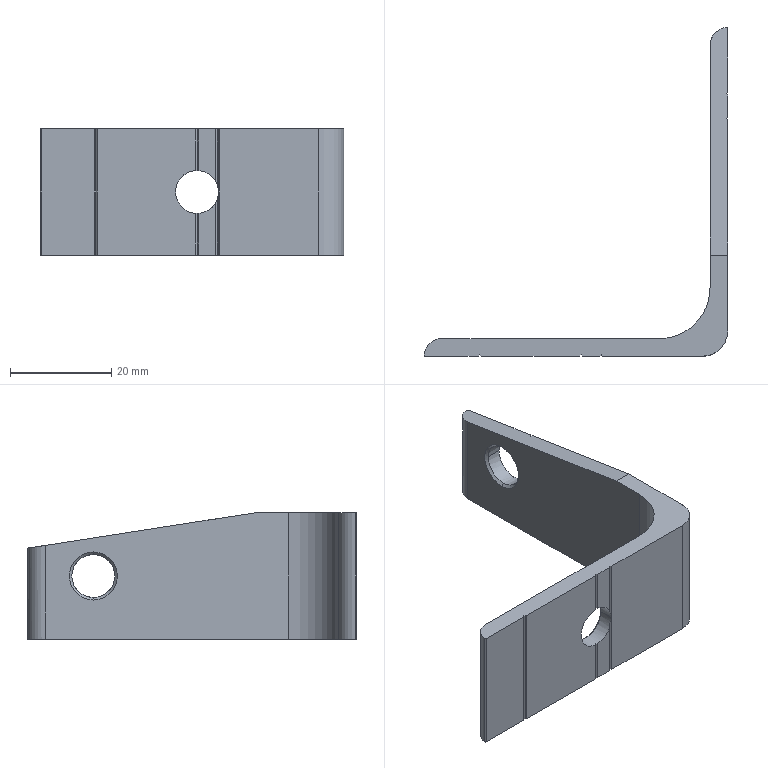Part | STEP file | V00-000000450 | 1 solid | 58 faces | box 60 x 64.996 x 25 mm | volume 9956 mm3 | plane 28 | cylinder 26 | cone 4 | commonest cylinder face diameters 0.2 x15 8.5 x4 0.4 x3 7 x2 10 x1 20 x1